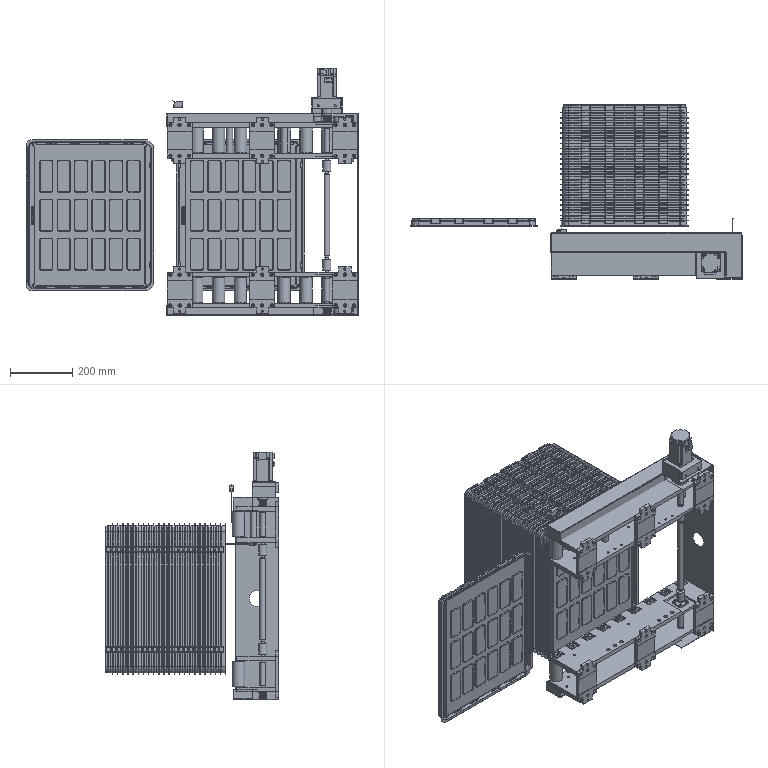Part | NX | 179 solids | 29969 faces | volume 18937016 mm3 | plane 13376 | cylinder 13187 | spline 2936 | cone 342 | torus 128 | commonest cylinder face diameters 10 x1962 13 x1769 3 x1539 0.3 x1040 0.56 x1040 3.95 x1040